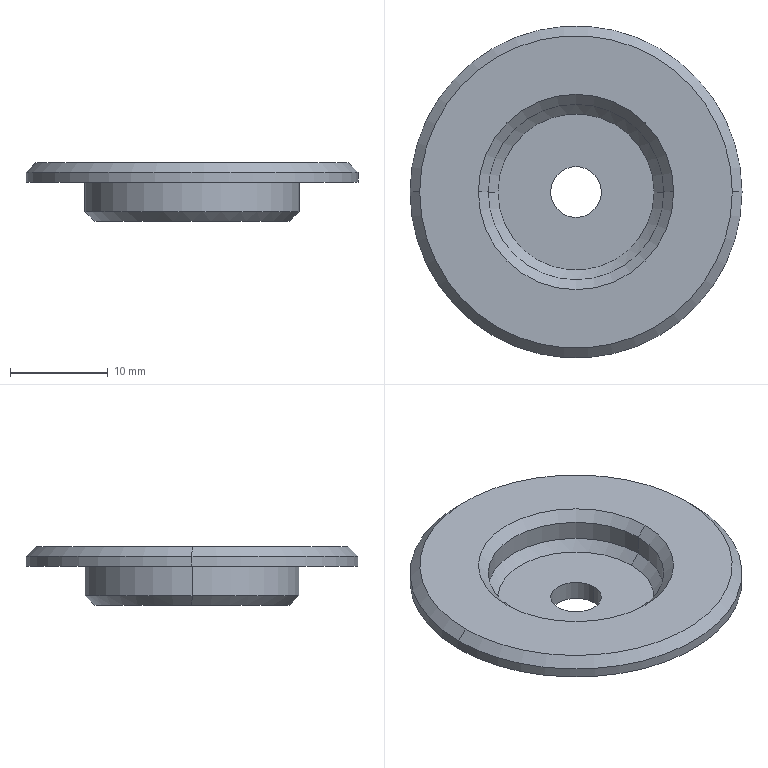Part | SolidWorks | features Chamfer 2, ICE 2, Extrusion 1 | 1 solid | 20 faces | box 34 x 34 x 6 mm | volume 2188 mm3 | cone 8 | cylinder 8 | plane 4 | commonest cylinder face diameters 5.2 x2 18 x2 22 x2 34 x2
STEP:
#1=CARTESIAN_POINT('',(-9.,0.,5.));
#2=VERTEX_POINT('',#1);
#3=CARTESIAN_POINT('',(9.,0.,5.));
#4=VERTEX_POINT('',#3);
#5=CARTESIAN_POINT('',(0.,0.,5.));
#6=DIRECTION('',(0.,0.,1.));
#7=DIRECTION('',(1.,0.,0.));
#8=AXIS2_PLACEMENT_3D('',#5,#6,#7);
#9=CIRCLE('',#8,9.);
#10=EDGE_CURVE('',#2,#4,#9,.T.);
#11=ORIENTED_EDGE('',*,*,#10,.F.);
#12=CARTESIAN_POINT('',(-10.,0.,6.));
#13=VERTEX_POINT('',#12);
#14=CARTESIAN_POINT('',(-9.,0.,5.));
#15=DIRECTION('',(-0.7071,0.,0.7071));
#16=VECTOR('',#15,1000.);
#17=LINE('',#14,#16);
#18=EDGE_CURVE('',#2,#13,#17,.T.);
#19=ORIENTED_EDGE('',*,*,#18,.T.);
#20=CARTESIAN_POINT('',(10.,0.,6.));
#21=VERTEX_POINT('',#20);
#22=CARTESIAN_POINT('',(0.,0.,6.));
#23=DIRECTION('',(0.,0.,-1.));
#24=DIRECTION('',(1.,0.,0.));
#25=AXIS2_PLACEMENT_3D('',#22,#23,#24);
#26=CIRCLE('',#25,10.);
#27=EDGE_CURVE('',#21,#13,#26,.T.);
#28=ORIENTED_EDGE('',*,*,#27,.F.);
#29=CARTESIAN_POINT('',(9.,0.,5.));
#30=DIRECTION('',(0.7071,0.,0.7071));
#31=VECTOR('',#30,1000.);
#32=LINE('',#29,#31);
#33=EDGE_CURVE('',#4,#21,#32,.T.);
#34=ORIENTED_EDGE('',*,*,#33,.F.);
#35=EDGE_LOOP('',(#11,#19,#28,#34));
#36=FACE_OUTER_BOUND('',#35,.T.);
#37=CARTESIAN_POINT('',(0.,0.,5.));
#38=DIRECTION('',(0.,0.,1.));
#39=DIRECTION('',(1.,0.,0.));
#40=AXIS2_PLACEMENT_3D('',#37,#38,#39);
#41=CONICAL_SURFACE('',#40,9.,0.7854);
#42=ADVANCED_FACE('',(#36),#41,.F.);
#43=CARTESIAN_POINT('',(16.,0.,6.));
#44=VERTEX_POINT('',#43);
#45=CARTESIAN_POINT('',(-16.,0.,6.));
#46=VERTEX_POINT('',#45);
#47=CARTESIAN_POINT('',(0.,0.,6.));
#48=DIRECTION('',(0.,0.,1.));
#49=DIRECTION('',(1.,0.,0.));
#50=AXIS2_PLACEMENT_3D('',#47,#48,#49);
#51=CIRCLE('',#50,16.);
#52=EDGE_CURVE('',#44,#46,#51,.T.);
#53=ORIENTED_EDGE('',*,*,#52,.F.);
#54=CARTESIAN_POINT('',(17.,0.,5.));
#55=VERTEX_POINT('',#54);
#56=CARTESIAN_POINT('',(16.,0.,6.));
#57=DIRECTION('',(0.7071,0.,-0.7071));
#58=VECTOR('',#57,1000.);
#59=LINE('',#56,#58);
#60=EDGE_CURVE('',#44,#55,#59,.T.);
#61=ORIENTED_EDGE('',*,*,#60,.T.);
#62=CARTESIAN_POINT('',(-17.,0.,5.));
#63=VERTEX_POINT('',#62);
#64=CARTESIAN_POINT('',(0.,0.,5.));
#65=DIRECTION('',(0.,0.,-1.));
#66=DIRECTION('',(1.,0.,0.));
#67=AXIS2_PLACEMENT_3D('',#64,#65,#66);
#68=CIRCLE('',#67,17.);
#69=EDGE_CURVE('',#63,#55,#68,.T.);
#70=ORIENTED_EDGE('',*,*,#69,.F.);
#71=CARTESIAN_POINT('',(-16.,0.,6.));
#72=DIRECTION('',(-0.7071,0.,-0.7071));
#73=VECTOR('',#72,1000.);
#74=LINE('',#71,#73);
#75=EDGE_CURVE('',#46,#63,#74,.T.);
#76=ORIENTED_EDGE('',*,*,#75,.F.);
#77=EDGE_LOOP('',(#53,#61,#70,#76));
#78=FACE_OUTER_BOUND('',#77,.T.);
#79=CARTESIAN_POINT('',(0.,0.,6.));
#80=DIRECTION('',(0.,0.,-1.));
#81=DIRECTION('',(-1.,0.,0.));
#82=AXIS2_PLACEMENT_3D('',#79,#80,#81);
#83=CONICAL_SURFACE('',#82,16.,0.7854);
#84=ADVANCED_FACE('',(#78),#83,.T.);
#85=CARTESIAN_POINT('',(17.,0.,4.));
#86=VERTEX_POINT('',#85);
#87=CARTESIAN_POINT('',(-17.,0.,4.));
#88=VERTEX_POINT('',#87);
#89=CARTESIAN_POINT('',(0.,0.,4.));
#90=DIRECTION('',(0.,0.,1.));
#91=DIRECTION('',(1.,0.,0.));
#92=AXIS2_PLACEMENT_3D('',#89,#90,#91);
#93=CIRCLE('',#92,17.);
#94=EDGE_CURVE('',#86,#88,#93,.T.);
#95=ORIENTED_EDGE('',*,*,#94,.T.);
#96=CARTESIAN_POINT('',(-17.,0.,4.));
#97=DIRECTION('',(0.,0.,1.));
#98=VECTOR('',#97,1000.);
#99=LINE('',#96,#98);
#100=EDGE_CURVE('',#88,#63,#99,.T.);
#101=ORIENTED_EDGE('',*,*,#100,.T.);
#102=ORIENTED_EDGE('',*,*,#69,.T.);
#103=CARTESIAN_POINT('',(17.,0.,4.));
#104=DIRECTION('',(0.,0.,1.));
#105=VECTOR('',#104,1000.);
#106=LINE('',#103,#105);
#107=EDGE_CURVE('',#86,#55,#106,.T.);
#108=ORIENTED_EDGE('',*,*,#107,.F.);
#109=EDGE_LOOP('',(#95,#101,#102,#108));
#110=FACE_OUTER_BOUND('',#109,.T.);
#111=CARTESIAN_POINT('',(0.,0.,4.));
#112=DIRECTION('',(0.,0.,1.));
#113=DIRECTION('',(1.,0.,0.));
#114=AXIS2_PLACEMENT_3D('',#111,#112,#113);
#115=CYLINDRICAL_SURFACE('',#114,17.);
#116=ADVANCED_FACE('',(#110),#115,.T.);
#117=CARTESIAN_POINT('',(-10.,0.,0.));
#118=VERTEX_POINT('',#117);
#119=CARTESIAN_POINT('',(10.,0.,0.));
#120=VERTEX_POINT('',#119);
#121=CARTESIAN_POINT('',(0.,0.,0.));
#122=DIRECTION('',(0.,0.,-1.));
#123=DIRECTION('',(1.,0.,0.));
#124=AXIS2_PLACEMENT_3D('',#121,#122,#123);
#125=CIRCLE('',#124,10.);
#126=EDGE_CURVE('',#118,#120,#125,.T.);
#127=ORIENTED_EDGE('',*,*,#126,.F.);
#128=CARTESIAN_POINT('',(-11.,0.,1.));
#129=VERTEX_POINT('',#128);
#130=CARTESIAN_POINT('',(-11.,0.,1.));
#131=DIRECTION('',(-0.7071,0.,0.7071));
#132=VECTOR('',#131,1000.);
#133=LINE('',#130,#132);
#134=EDGE_CURVE('',#118,#129,#133,.T.);
#135=ORIENTED_EDGE('',*,*,#134,.T.);
#136=CARTESIAN_POINT('',(11.,0.,1.));
#137=VERTEX_POINT('',#136);
#138=CARTESIAN_POINT('',(0.,0.,1.));
#139=DIRECTION('',(0.,0.,1.));
#140=DIRECTION('',(1.,0.,0.));
#141=AXIS2_PLACEMENT_3D('',#138,#139,#140);
#142=CIRCLE('',#141,11.);
#143=EDGE_CURVE('',#137,#129,#142,.T.);
#144=ORIENTED_EDGE('',*,*,#143,.F.);
#145=CARTESIAN_POINT('',(11.,0.,1.));
#146=DIRECTION('',(0.7071,0.,0.7071));
#147=VECTOR('',#146,1000.);
#148=LINE('',#145,#147);
#149=EDGE_CURVE('',#120,#137,#148,.T.);
#150=ORIENTED_EDGE('',*,*,#149,.F.);
#151=EDGE_LOOP('',(#127,#135,#144,#150));
#152=FACE_OUTER_BOUND('',#151,.T.);
#153=CARTESIAN_POINT('',(0.,0.,1.));
#154=DIRECTION('',(0.,0.,1.));
#155=DIRECTION('',(1.,0.,0.));
#156=AXIS2_PLACEMENT_3D('',#153,#154,#155);
#157=CONICAL_SURFACE('',#156,11.,0.7854);
#158=ADVANCED_FACE('',(#152),#157,.T.);
#159=CARTESIAN_POINT('',(-8.,0.,2.));
#160=VERTEX_POINT('',#159);
#161=CARTESIAN_POINT('',(8.,0.,2.));
#162=VERTEX_POINT('',#161);
#163=CARTESIAN_POINT('',(0.,0.,2.));
#164=DIRECTION('',(0.,0.,1.));
#165=DIRECTION('',(-1.,0.,0.));
#166=AXIS2_PLACEMENT_3D('',#163,#164,#165);
#167=CIRCLE('',#166,8.);
#168=EDGE_CURVE('',#160,#162,#167,.T.);
#169=ORIENTED_EDGE('',*,*,#168,.F.);
#170=CARTESIAN_POINT('',(-9.,0.,3.));
#171=VERTEX_POINT('',#170);
#172=CARTESIAN_POINT('',(-9.,0.,3.));
#173=DIRECTION('',(-0.7071,0.,0.7071));
#174=VECTOR('',#173,1000.);
#175=LINE('',#172,#174);
#176=EDGE_CURVE('',#160,#171,#175,.T.);
#177=ORIENTED_EDGE('',*,*,#176,.T.);
#178=CARTESIAN_POINT('',(9.,0.,3.));
#179=VERTEX_POINT('',#178);
#180=CARTESIAN_POINT('',(0.,0.,3.));
#181=DIRECTION('',(0.,0.,-1.));
#182=DIRECTION('',(-1.,0.,0.));
#183=AXIS2_PLACEMENT_3D('',#180,#181,#182);
#184=CIRCLE('',#183,9.);
#185=EDGE_CURVE('',#179,#171,#184,.T.);
#186=ORIENTED_EDGE('',*,*,#185,.F.);
#187=CARTESIAN_POINT('',(9.,0.,3.));
#188=DIRECTION('',(0.7071,0.,0.7071));
#189=VECTOR('',#188,1000.);
#190=LINE('',#187,#189);
#191=EDGE_CURVE('',#162,#179,#190,.T.);
#192=ORIENTED_EDGE('',*,*,#191,.F.);
#193=EDGE_LOOP('',(#169,#177,#186,#192));
#194=FACE_OUTER_BOUND('',#193,.T.);
#195=CARTESIAN_POINT('',(0.,0.,3.));
#196=DIRECTION('',(0.,0.,1.));
#197=DIRECTION('',(1.,0.,0.));
#198=AXIS2_PLACEMENT_3D('',#195,#196,#197);
#199=CONICAL_SURFACE('',#198,9.,0.7854);
#200=ADVANCED_FACE('',(#194),#199,.F.);
#201=CARTESIAN_POINT('',(2.6,0.,2.));
#202=VERTEX_POINT('',#201);
#203=CARTESIAN_POINT('',(-2.6,0.,2.));
#204=VERTEX_POINT('',#203);
#205=CARTESIAN_POINT('',(0.,0.,2.));
#206=DIRECTION('',(0.,0.,-1.));
#207=DIRECTION('',(-1.,0.,0.));
#208=AXIS2_PLACEMENT_3D('',#205,#206,#207);
#209=CIRCLE('',#208,2.6);
#210=EDGE_CURVE('',#202,#204,#209,.T.);
#211=ORIENTED_EDGE('',*,*,#210,.F.);
#212=CARTESIAN_POINT('',(2.6,0.,0.));
#213=VERTEX_POINT('',#212);
#214=CARTESIAN_POINT('',(2.6,0.,2.));
#215=DIRECTION('',(0.,0.,-1.));
#216=VECTOR('',#215,1000.);
#217=LINE('',#214,#216);
#218=EDGE_CURVE('',#202,#213,#217,.T.);
#219=ORIENTED_EDGE('',*,*,#218,.T.);
#220=CARTESIAN_POINT('',(-2.6,0.,0.));
#221=VERTEX_POINT('',#220);
#222=CARTESIAN_POINT('',(0.,0.,0.));
#223=DIRECTION('',(0.,0.,-1.));
#224=DIRECTION('',(-1.,0.,0.));
#225=AXIS2_PLACEMENT_3D('',#222,#223,#224);
#226=CIRCLE('',#225,2.6);
#227=EDGE_CURVE('',#213,#221,#226,.T.);
#228=ORIENTED_EDGE('',*,*,#227,.T.);
#229=CARTESIAN_POINT('',(-2.6,0.,2.));
#230=DIRECTION('',(0.,0.,-1.));
#231=VECTOR('',#230,1000.);
#232=LINE('',#229,#231);
#233=EDGE_CURVE('',#204,#221,#232,.T.);
#234=ORIENTED_EDGE('',*,*,#233,.F.);
#235=EDGE_LOOP('',(#211,#219,#228,#234));
#236=FACE_OUTER_BOUND('',#235,.T.);
#237=CARTESIAN_POINT('',(0.,0.,2.));
#238=DIRECTION('',(0.,0.,-1.));
#239=DIRECTION('',(-1.,0.,0.));
#240=AXIS2_PLACEMENT_3D('',#237,#238,#239);
#241=CYLINDRICAL_SURFACE('',#240,2.6);
#242=ADVANCED_FACE('',(#236),#241,.F.);
#243=ORIENTED_EDGE('',*,*,#10,.T.);
#244=CARTESIAN_POINT('',(9.,0.,6.));
#245=DIRECTION('',(0.,0.,-1.));
#246=VECTOR('',#245,1000.);
#247=LINE('',#244,#246);
#248=EDGE_CURVE('',#4,#179,#247,.T.);
#249=ORIENTED_EDGE('',*,*,#248,.T.);
#250=ORIENTED_EDGE('',*,*,#185,.T.);
#251=CARTESIAN_POINT('',(-9.,0.,6.));
#252=DIRECTION('',(0.,0.,-1.));
#253=VECTOR('',#252,1000.);
#254=LINE('',#251,#253);
#255=EDGE_CURVE('',#2,#171,#254,.T.);
#256=ORIENTED_EDGE('',*,*,#255,.F.);
#257=EDGE_LOOP('',(#243,#249,#250,#256));
#258=FACE_OUTER_BOUND('',#257,.T.);
#259=CARTESIAN_POINT('',(0.,0.,6.));
#260=DIRECTION('',(0.,0.,-1.));
#261=DIRECTION('',(-1.,0.,0.));
#262=AXIS2_PLACEMENT_3D('',#259,#260,#261);
#263=CYLINDRICAL_SURFACE('',#262,9.);
#264=ADVANCED_FACE('',(#258),#263,.F.);
#265=CARTESIAN_POINT('',(11.,0.,4.));
#266=VERTEX_POINT('',#265);
#267=CARTESIAN_POINT('',(-11.,0.,4.));
#268=VERTEX_POINT('',#267);
#269=CARTESIAN_POINT('',(0.,0.,4.));
#270=DIRECTION('',(0.,0.,1.));
#271=DIRECTION('',(1.,0.,0.));
#272=AXIS2_PLACEMENT_3D('',#269,#270,#271);
#273=CIRCLE('',#272,11.);
#274=EDGE_CURVE('',#266,#268,#273,.T.);
#275=ORIENTED_EDGE('',*,*,#274,.F.);
#276=CARTESIAN_POINT('',(11.,0.,6.));
#277=DIRECTION('',(0.,0.,-1.));
#278=VECTOR('',#277,1000.);
#279=LINE('',#276,#278);
#280=EDGE_CURVE('',#266,#137,#279,.T.);
#281=ORIENTED_EDGE('',*,*,#280,.T.);
#282=ORIENTED_EDGE('',*,*,#143,.T.);
#283=CARTESIAN_POINT('',(-11.,0.,6.));
#284=DIRECTION('',(0.,0.,-1.));
#285=VECTOR('',#284,1000.);
#286=LINE('',#283,#285);
#287=EDGE_CURVE('',#268,#129,#286,.T.);
#288=ORIENTED_EDGE('',*,*,#287,.F.);
#289=EDGE_LOOP('',(#275,#281,#282,#288));
#290=FACE_OUTER_BOUND('',#289,.T.);
#291=CARTESIAN_POINT('',(0.,0.,6.));
#292=DIRECTION('',(0.,0.,-1.));
#293=DIRECTION('',(-1.,0.,0.));
#294=AXIS2_PLACEMENT_3D('',#291,#292,#293);
#295=CYLINDRICAL_SURFACE('',#294,11.);
#296=ADVANCED_FACE('',(#290),#295,.T.);
#297=ORIENTED_EDGE('',*,*,#280,.F.);
#298=CARTESIAN_POINT('',(0.,0.,4.));
#299=DIRECTION('',(0.,0.,1.));
#300=DIRECTION('',(1.,0.,0.));
#301=AXIS2_PLACEMENT_3D('',#298,#299,#300);
#302=CIRCLE('',#301,11.);
#303=EDGE_CURVE('',#268,#266,#302,.T.);
#304=ORIENTED_EDGE('',*,*,#303,.F.);
#305=ORIENTED_EDGE('',*,*,#287,.T.);
#306=CARTESIAN_POINT('',(0.,0.,1.));
#307=DIRECTION('',(0.,0.,1.));
#308=DIRECTION('',(1.,0.,0.));
#309=AXIS2_PLACEMENT_3D('',#306,#307,#308);
#310=CIRCLE('',#309,11.);
#311=EDGE_CURVE('',#129,#137,#310,.T.);
#312=ORIENTED_EDGE('',*,*,#311,.T.);
#313=EDGE_LOOP('',(#297,#304,#305,#312));
#314=FACE_OUTER_BOUND('',#313,.T.);
#315=CARTESIAN_POINT('',(0.,0.,6.));
#316=DIRECTION('',(0.,0.,-1.));
#317=DIRECTION('',(-1.,0.,0.));
#318=AXIS2_PLACEMENT_3D('',#315,#316,#317);
#319=CYLINDRICAL_SURFACE('',#318,11.);
#320=ADVANCED_FACE('',(#314),#319,.T.);
#321=ORIENTED_EDGE('',*,*,#248,.F.);
#322=CARTESIAN_POINT('',(0.,0.,5.));
#323=DIRECTION('',(0.,0.,1.));
#324=DIRECTION('',(1.,0.,0.));
#325=AXIS2_PLACEMENT_3D('',#322,#323,#324);
#326=CIRCLE('',#325,9.);
#327=EDGE_CURVE('',#4,#2,#326,.T.);
#328=ORIENTED_EDGE('',*,*,#327,.T.);
#329=ORIENTED_EDGE('',*,*,#255,.T.);
#330=CARTESIAN_POINT('',(0.,0.,3.));
#331=DIRECTION('',(0.,0.,-1.));
#332=DIRECTION('',(-1.,0.,0.));
#333=AXIS2_PLACEMENT_3D('',#330,#331,#332);
#334=CIRCLE('',#333,9.);
#335=EDGE_CURVE('',#171,#179,#334,.T.);
#336=ORIENTED_EDGE('',*,*,#335,.T.);
#337=EDGE_LOOP('',(#321,#328,#329,#336));
#338=FACE_OUTER_BOUND('',#337,.T.);
#339=CARTESIAN_POINT('',(0.,0.,6.));
#340=DIRECTION('',(0.,0.,-1.));
#341=DIRECTION('',(-1.,0.,0.));
#342=AXIS2_PLACEMENT_3D('',#339,#340,#341);
#343=CYLINDRICAL_SURFACE('',#342,9.);
#344=ADVANCED_FACE('',(#338),#343,.F.);
#345=CARTESIAN_POINT('',(0.,0.,6.));
#346=DIRECTION('',(0.,0.,1.));
#347=DIRECTION('',(1.,0.,0.));
#348=AXIS2_PLACEMENT_3D('',#345,#346,#347);
#349=CIRCLE('',#348,16.);
#350=EDGE_CURVE('',#46,#44,#349,.T.);
#351=ORIENTED_EDGE('',*,*,#350,.T.);
#352=ORIENTED_EDGE('',*,*,#52,.T.);
#353=EDGE_LOOP('',(#351,#352));
#354=FACE_OUTER_BOUND('',#353,.T.);
#355=ORIENTED_EDGE('',*,*,#27,.T.);
#356=CARTESIAN_POINT('',(0.,0.,6.));
#357=DIRECTION('',(0.,0.,-1.));
#358=DIRECTION('',(1.,0.,0.));
#359=AXIS2_PLACEMENT_3D('',#356,#357,#358);
#360=CIRCLE('',#359,10.);
#361=EDGE_CURVE('',#13,#21,#360,.T.);
#362=ORIENTED_EDGE('',*,*,#361,.T.);
#363=EDGE_LOOP('',(#355,#362));
#364=FACE_BOUND('',#363,.T.);
#365=CARTESIAN_POINT('',(0.,0.,6.));
#366=DIRECTION('',(0.,0.,1.));
#367=DIRECTION('',(1.,0.,0.));
#368=AXIS2_PLACEMENT_3D('',#365,#366,#367);
#369=PLANE('',#368);
#370=ADVANCED_FACE('',(#354,#364),#369,.T.);
#371=CARTESIAN_POINT('',(0.,0.,0.));
#372=DIRECTION('',(0.,0.,-1.));
#373=DIRECTION('',(1.,0.,0.));
#374=AXIS2_PLACEMENT_3D('',#371,#372,#373);
#375=CIRCLE('',#374,10.);
#376=EDGE_CURVE('',#120,#118,#375,.T.);
#377=ORIENTED_EDGE('',*,*,#376,.T.);
#378=ORIENTED_EDGE('',*,*,#126,.T.);
#379=EDGE_LOOP('',(#377,#378));
#380=FACE_OUTER_BOUND('',#379,.T.);
#381=CARTESIAN_POINT('',(0.,0.,0.));
#382=DIRECTION('',(0.,0.,-1.));
#383=DIRECTION('',(-1.,0.,0.));
#384=AXIS2_PLACEMENT_3D('',#381,#382,#383);
#385=CIRCLE('',#384,2.6);
#386=EDGE_CURVE('',#221,#213,#385,.T.);
#387=ORIENTED_EDGE('',*,*,#386,.F.);
#388=ORIENTED_EDGE('',*,*,#227,.F.);
#389=EDGE_LOOP('',(#387,#388));
#390=FACE_BOUND('',#389,.T.);
#391=CARTESIAN_POINT('',(0.,0.,0.));
#392=DIRECTION('',(0.,0.,1.));
#393=DIRECTION('',(1.,0.,0.));
#394=AXIS2_PLACEMENT_3D('',#391,#392,#393);
#395=PLANE('',#394);
#396=ADVANCED_FACE('',(#380,#390),#395,.F.);
#397=CARTESIAN_POINT('',(0.,0.,2.));
#398=DIRECTION('',(0.,0.,1.));
#399=DIRECTION('',(-1.,0.,0.));
#400=AXIS2_PLACEMENT_3D('',#397,#398,#399);
#401=CIRCLE('',#400,8.);
#402=EDGE_CURVE('',#162,#160,#401,.T.);
#403=ORIENTED_EDGE('',*,*,#402,.T.);
#404=ORIENTED_EDGE('',*,*,#168,.T.);
#405=EDGE_LOOP('',(#403,#404));
#406=FACE_OUTER_BOUND('',#405,.T.);
#407=CARTESIAN_POINT('',(0.,0.,2.));
#408=DIRECTION('',(0.,0.,-1.));
#409=DIRECTION('',(-1.,0.,0.));
#410=AXIS2_PLACEMENT_3D('',#407,#408,#409);
#411=CIRCLE('',#410,2.6);
#412=EDGE_CURVE('',#204,#202,#411,.T.);
#413=ORIENTED_EDGE('',*,*,#412,.T.);
#414=ORIENTED_EDGE('',*,*,#210,.T.);
#415=EDGE_LOOP('',(#413,#414));
#416=FACE_BOUND('',#415,.T.);
#417=CARTESIAN_POINT('',(0.,0.,2.));
#418=DIRECTION('',(0.,0.,-1.));
#419=DIRECTION('',(-1.,0.,0.));
#420=AXIS2_PLACEMENT_3D('',#417,#418,#419);
#421=PLANE('',#420);
#422=ADVANCED_FACE('',(#406,#416),#421,.F.);
#423=ORIENTED_EDGE('',*,*,#218,.F.);
#424=ORIENTED_EDGE('',*,*,#412,.F.);
#425=ORIENTED_EDGE('',*,*,#233,.T.);
#426=ORIENTED_EDGE('',*,*,#386,.T.);
#427=EDGE_LOOP('',(#423,#424,#425,#426));
#428=FACE_OUTER_BOUND('',#427,.T.);
#429=CARTESIAN_POINT('',(0.,0.,2.));
#430=DIRECTION('',(0.,0.,-1.));
#431=DIRECTION('',(-1.,0.,0.));
#432=AXIS2_PLACEMENT_3D('',#429,#430,#431);
#433=CYLINDRICAL_SURFACE('',#432,2.6);
#434=ADVANCED_FACE('',(#428),#433,.F.);
#435=ORIENTED_EDGE('',*,*,#176,.F.);
#436=ORIENTED_EDGE('',*,*,#402,.F.);
#437=ORIENTED_EDGE('',*,*,#191,.T.);
#438=ORIENTED_EDGE('',*,*,#335,.F.);
#439=EDGE_LOOP('',(#435,#436,#437,#438));
#440=FACE_OUTER_BOUND('',#439,.T.);
#441=CARTESIAN_POINT('',(0.,0.,3.));
#442=DIRECTION('',(0.,0.,1.));
#443=DIRECTION('',(1.,0.,0.));
#444=AXIS2_PLACEMENT_3D('',#441,#442,#443);
#445=CONICAL_SURFACE('',#444,9.,0.7854);
#446=ADVANCED_FACE('',(#440),#445,.F.);
#447=ORIENTED_EDGE('',*,*,#134,.F.);
#448=ORIENTED_EDGE('',*,*,#376,.F.);
#449=ORIENTED_EDGE('',*,*,#149,.T.);
#450=ORIENTED_EDGE('',*,*,#311,.F.);
#451=EDGE_LOOP('',(#447,#448,#449,#450));
#452=FACE_OUTER_BOUND('',#451,.T.);
#453=CARTESIAN_POINT('',(0.,0.,1.));
#454=DIRECTION('',(0.,0.,1.));
#455=DIRECTION('',(1.,0.,0.));
#456=AXIS2_PLACEMENT_3D('',#453,#454,#455);
#457=CONICAL_SURFACE('',#456,11.,0.7854);
#458=ADVANCED_FACE('',(#452),#457,.T.);
#459=ORIENTED_EDGE('',*,*,#100,.F.);
#460=CARTESIAN_POINT('',(0.,0.,4.));
#461=DIRECTION('',(0.,0.,1.));
#462=DIRECTION('',(1.,0.,0.));
#463=AXIS2_PLACEMENT_3D('',#460,#461,#462);
#464=CIRCLE('',#463,17.);
#465=EDGE_CURVE('',#88,#86,#464,.T.);
#466=ORIENTED_EDGE('',*,*,#465,.T.);
#467=ORIENTED_EDGE('',*,*,#107,.T.);
#468=CARTESIAN_POINT('',(0.,0.,5.));
#469=DIRECTION('',(0.,0.,-1.));
#470=DIRECTION('',(1.,0.,0.));
#471=AXIS2_PLACEMENT_3D('',#468,#469,#470);
#472=CIRCLE('',#471,17.);
#473=EDGE_CURVE('',#55,#63,#472,.T.);
#474=ORIENTED_EDGE('',*,*,#473,.T.);
#475=EDGE_LOOP('',(#459,#466,#467,#474));
#476=FACE_OUTER_BOUND('',#475,.T.);
#477=CARTESIAN_POINT('',(0.,0.,4.));
#478=DIRECTION('',(0.,0.,1.));
#479=DIRECTION('',(1.,0.,0.));
#480=AXIS2_PLACEMENT_3D('',#477,#478,#479);
#481=CYLINDRICAL_SURFACE('',#480,17.);
#482=ADVANCED_FACE('',(#476),#481,.T.);
#483=ORIENTED_EDGE('',*,*,#303,.T.);
#484=ORIENTED_EDGE('',*,*,#274,.T.);
#485=EDGE_LOOP('',(#483,#484));
#486=FACE_BOUND('',#485,.T.);
#487=ORIENTED_EDGE('',*,*,#94,.F.);
#488=ORIENTED_EDGE('',*,*,#465,.F.);
#489=EDGE_LOOP('',(#487,#488));
#490=FACE_OUTER_BOUND('',#489,.T.);
#491=CARTESIAN_POINT('',(0.,0.,4.));
#492=DIRECTION('',(0.,0.,1.));
#493=DIRECTION('',(1.,0.,0.));
#494=AXIS2_PLACEMENT_3D('',#491,#492,#493);
#495=PLANE('',#494);
#496=ADVANCED_FACE('',(#486,#490),#495,.F.);
#497=ORIENTED_EDGE('',*,*,#60,.F.);
#498=ORIENTED_EDGE('',*,*,#350,.F.);
#499=ORIENTED_EDGE('',*,*,#75,.T.);
#500=ORIENTED_EDGE('',*,*,#473,.F.);
#501=EDGE_LOOP('',(#497,#498,#499,#500));
#502=FACE_OUTER_BOUND('',#501,.T.);
#503=CARTESIAN_POINT('',(0.,0.,6.));
#504=DIRECTION('',(0.,0.,-1.));
#505=DIRECTION('',(-1.,0.,0.));
#506=AXIS2_PLACEMENT_3D('',#503,#504,#505);
#507=CONICAL_SURFACE('',#506,16.,0.7854);
#508=ADVANCED_FACE('',(#502),#507,.T.);
#509=ORIENTED_EDGE('',*,*,#18,.F.);
#510=ORIENTED_EDGE('',*,*,#327,.F.);
#511=ORIENTED_EDGE('',*,*,#33,.T.);
#512=ORIENTED_EDGE('',*,*,#361,.F.);
#513=EDGE_LOOP('',(#509,#510,#511,#512));
#514=FACE_OUTER_BOUND('',#513,.T.);
#515=CARTESIAN_POINT('',(0.,0.,5.));
#516=DIRECTION('',(0.,0.,1.));
#517=DIRECTION('',(1.,0.,0.));
#518=AXIS2_PLACEMENT_3D('',#515,#516,#517);
#519=CONICAL_SURFACE('',#518,9.,0.7854);
#520=ADVANCED_FACE('',(#514),#519,.F.);
#521=CLOSED_SHELL('',(#42,#84,#116,#158,#200,#242,#264,#296,#320,#344,#370,#396,#422,#434,#446,#458,#482,#496,#508,#520));
#522=MANIFOLD_SOLID_BREP('',#521);
#523=CARTESIAN_POINT('',(0.,0.,0.));
#524=DIRECTION('',(0.,0.,1.));
#525=DIRECTION('',(1.,0.,0.));
#526=AXIS2_PLACEMENT_3D('',#523,#524,#525);
#527=(LENGTH_UNIT()NAMED_UNIT(*)SI_UNIT(.MILLI.,.METRE.));
#528=UNCERTAINTY_MEASURE_WITH_UNIT(LENGTH_MEASURE(0.00001),#527,'','');
#529=(NAMED_UNIT(*)PLANE_ANGLE_UNIT()SI_UNIT($,.RADIAN.));
#530=(NAMED_UNIT(*)SI_UNIT($,.STERADIAN.)SOLID_ANGLE_UNIT());
#531=(GEOMETRIC_REPRESENTATION_CONTEXT(3)GLOBAL_UNCERTAINTY_ASSIGNED_CONTEXT((#528))GLOBAL_UNIT_ASSIGNED_CONTEXT((#527,#529,#530))REPRESENTATION_CONTEXT('',''));
#532=ADVANCED_BREP_SHAPE_REPRESENTATION('',(#522,#526),#531);